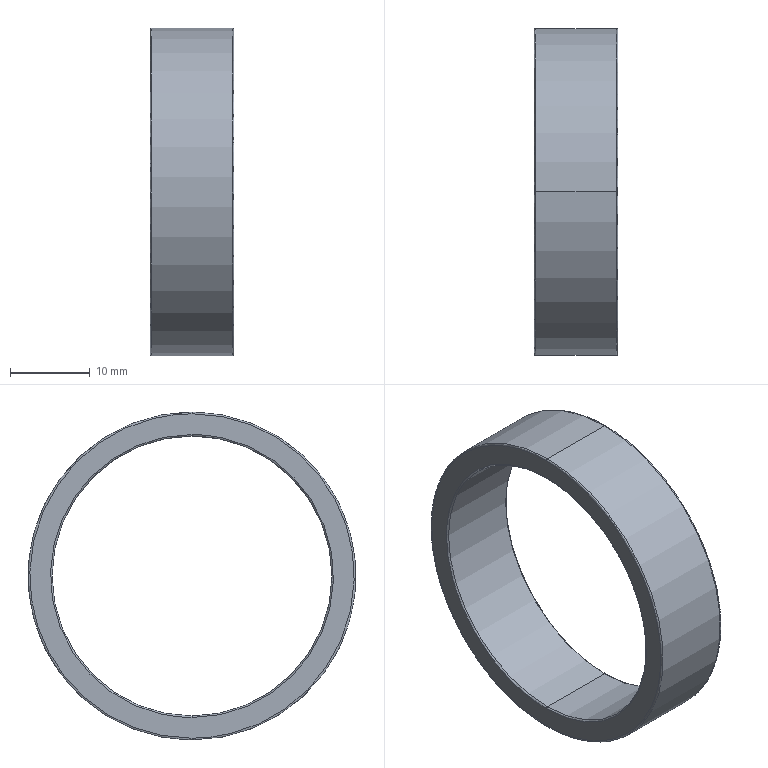Part | SolidWorks | features BaseBody 1 | 1 solid | 14 faces | box 10.5 x 41 x 41 mm | volume 3744 mm3 | spline 8 | cylinder 4 | plane 2 | commonest cylinder face diameters 35.02 x2 41 x2
STEP:
#1=CARTESIAN_POINT('',(10.3,-0.000000002,-20.5));
#2=VERTEX_POINT('',#1);
#3=CARTESIAN_POINT('',(10.3,0.,20.5));
#4=VERTEX_POINT('',#3);
#5=CARTESIAN_POINT('',(10.3,0.,0.));
#6=DIRECTION('',(1.,0.,0.));
#7=DIRECTION('',(0.,1.,0.));
#8=AXIS2_PLACEMENT_3D('',#5,#6,#7);
#9=CIRCLE('',#8,20.5);
#10=EDGE_CURVE('',#2,#4,#9,.T.);
#11=ORIENTED_EDGE('',*,*,#10,.F.);
#12=CARTESIAN_POINT('',(0.2,-0.000000002,-20.5));
#13=VERTEX_POINT('',#12);
#14=CARTESIAN_POINT('',(10.3,0.,-20.5));
#15=DIRECTION('',(-1.,0.,0.));
#16=VECTOR('',#15,1000.);
#17=LINE('',#14,#16);
#18=EDGE_CURVE('',#2,#13,#17,.T.);
#19=ORIENTED_EDGE('',*,*,#18,.T.);
#20=CARTESIAN_POINT('',(0.2,-0.000000001,20.5));
#21=VERTEX_POINT('',#20);
#22=CARTESIAN_POINT('',(0.2,0.,0.));
#23=DIRECTION('',(-1.,0.,0.));
#24=DIRECTION('',(0.,0.,1.));
#25=AXIS2_PLACEMENT_3D('',#22,#23,#24);
#26=CIRCLE('',#25,20.5);
#27=EDGE_CURVE('',#21,#13,#26,.T.);
#28=ORIENTED_EDGE('',*,*,#27,.F.);
#29=CARTESIAN_POINT('',(10.3,0.,20.5));
#30=DIRECTION('',(-1.,0.,0.));
#31=VECTOR('',#30,1000.);
#32=LINE('',#29,#31);
#33=EDGE_CURVE('',#4,#21,#32,.T.);
#34=ORIENTED_EDGE('',*,*,#33,.F.);
#35=EDGE_LOOP('',(#11,#19,#28,#34));
#36=FACE_OUTER_BOUND('',#35,.T.);
#37=CARTESIAN_POINT('',(10.3,0.,0.));
#38=DIRECTION('',(-1.,0.,0.));
#39=DIRECTION('',(0.,0.,1.));
#40=AXIS2_PLACEMENT_3D('',#37,#38,#39);
#41=CYLINDRICAL_SURFACE('',#40,20.5);
#42=ADVANCED_FACE('',(#36),#41,.T.);
#43=CARTESIAN_POINT('',(10.3,-0.000000002,-17.51));
#44=VERTEX_POINT('',#43);
#45=CARTESIAN_POINT('',(10.3,0.,17.51));
#46=VERTEX_POINT('',#45);
#47=CARTESIAN_POINT('',(10.3,0.,0.));
#48=DIRECTION('',(-1.,0.,0.));
#49=DIRECTION('',(0.,-1.,0.));
#50=AXIS2_PLACEMENT_3D('',#47,#48,#49);
#51=CIRCLE('',#50,17.51);
#52=EDGE_CURVE('',#44,#46,#51,.T.);
#53=ORIENTED_EDGE('',*,*,#52,.F.);
#54=CARTESIAN_POINT('',(0.2,-0.000000004,-17.51));
#55=VERTEX_POINT('',#54);
#56=CARTESIAN_POINT('',(10.3,0.,-17.51));
#57=DIRECTION('',(-1.,0.,0.));
#58=VECTOR('',#57,1000.);
#59=LINE('',#56,#58);
#60=EDGE_CURVE('',#44,#55,#59,.T.);
#61=ORIENTED_EDGE('',*,*,#60,.T.);
#62=CARTESIAN_POINT('',(0.2,0.,17.51));
#63=VERTEX_POINT('',#62);
#64=CARTESIAN_POINT('',(0.2,0.,0.));
#65=DIRECTION('',(-1.,0.,0.));
#66=DIRECTION('',(0.,0.,1.));
#67=AXIS2_PLACEMENT_3D('',#64,#65,#66);
#68=CIRCLE('',#67,17.51);
#69=EDGE_CURVE('',#55,#63,#68,.T.);
#70=ORIENTED_EDGE('',*,*,#69,.T.);
#71=CARTESIAN_POINT('',(10.3,0.,17.51));
#72=DIRECTION('',(-1.,0.,0.));
#73=VECTOR('',#72,1000.);
#74=LINE('',#71,#73);
#75=EDGE_CURVE('',#46,#63,#74,.T.);
#76=ORIENTED_EDGE('',*,*,#75,.F.);
#77=EDGE_LOOP('',(#53,#61,#70,#76));
#78=FACE_OUTER_BOUND('',#77,.T.);
#79=CARTESIAN_POINT('',(10.3,0.,0.));
#80=DIRECTION('',(-1.,0.,0.));
#81=DIRECTION('',(0.,0.,1.));
#82=AXIS2_PLACEMENT_3D('',#79,#80,#81);
#83=CYLINDRICAL_SURFACE('',#82,17.51);
#84=ADVANCED_FACE('',(#78),#83,.F.);
#85=CARTESIAN_POINT('',(10.5,0.,20.3));
#86=VERTEX_POINT('',#85);
#87=CARTESIAN_POINT('',(10.5,0.,-20.3));
#88=VERTEX_POINT('',#87);
#89=CARTESIAN_POINT('',(10.5,0.,20.3));
#90=CARTESIAN_POINT('',(10.5,40.6,20.3));
#91=CARTESIAN_POINT('',(10.5,40.6,-20.3));
#92=CARTESIAN_POINT('',(10.5,0.,-20.3));
#93=(BOUNDED_CURVE()B_SPLINE_CURVE(3,(#89,#90,#91,#92),.UNSPECIFIED.,.F.,.F.)B_SPLINE_CURVE_WITH_KNOTS((4,4),(0.,1.),.UNSPECIFIED.)CURVE()GEOMETRIC_REPRESENTATION_ITEM()RATIONAL_B_SPLINE_CURVE((0.9566,0.3189,0.3189,0.9566))REPRESENTATION_ITEM(''));
#94=EDGE_CURVE('',#86,#88,#93,.T.);
#95=ORIENTED_EDGE('',*,*,#94,.T.);
#96=CARTESIAN_POINT('',(10.3,-0.000000002,-20.5));
#97=CARTESIAN_POINT('',(10.417,0.,-20.5));
#98=CARTESIAN_POINT('',(10.5,0.,-20.417));
#99=CARTESIAN_POINT('',(10.5,0.,-20.3));
#100=(BOUNDED_CURVE()B_SPLINE_CURVE(3,(#96,#97,#98,#99),.UNSPECIFIED.,.F.,.F.)B_SPLINE_CURVE_WITH_KNOTS((4,4),(0.06314,0.9369),.UNSPECIFIED.)CURVE()GEOMETRIC_REPRESENTATION_ITEM()RATIONAL_B_SPLINE_CURVE((0.9566,0.7698,0.7698,0.9566))REPRESENTATION_ITEM(''));
#101=EDGE_CURVE('',#2,#88,#100,.T.);
#102=ORIENTED_EDGE('',*,*,#101,.F.);
#103=ORIENTED_EDGE('',*,*,#10,.T.);
#104=CARTESIAN_POINT('',(10.5,0.,20.3));
#105=CARTESIAN_POINT('',(10.5,0.,20.417));
#106=CARTESIAN_POINT('',(10.417,0.,20.5));
#107=CARTESIAN_POINT('',(10.3,0.,20.5));
#108=(BOUNDED_CURVE()B_SPLINE_CURVE(3,(#104,#105,#106,#107),.UNSPECIFIED.,.F.,.F.)B_SPLINE_CURVE_WITH_KNOTS((4,4),(0.06314,0.9369),.UNSPECIFIED.)CURVE()GEOMETRIC_REPRESENTATION_ITEM()RATIONAL_B_SPLINE_CURVE((0.9566,0.7698,0.7698,0.9566))REPRESENTATION_ITEM(''));
#109=EDGE_CURVE('',#86,#4,#108,.T.);
#110=ORIENTED_EDGE('',*,*,#109,.F.);
#111=EDGE_LOOP('',(#95,#102,#103,#110));
#112=FACE_OUTER_BOUND('',#111,.T.);
#113=CARTESIAN_POINT('',(10.499,0.,-20.28));
#114=CARTESIAN_POINT('',(10.499,40.56,-20.28));
#115=CARTESIAN_POINT('',(10.499,40.56,20.28));
#116=CARTESIAN_POINT('',(10.499,0.,20.28));
#117=CARTESIAN_POINT('',(10.513,0.,-20.416));
#118=CARTESIAN_POINT('',(10.513,40.832,-20.416));
#119=CARTESIAN_POINT('',(10.513,40.832,20.416));
#120=CARTESIAN_POINT('',(10.513,0.,20.416));
#121=CARTESIAN_POINT('',(10.416,0.,-20.513));
#122=CARTESIAN_POINT('',(10.416,41.025,-20.513));
#123=CARTESIAN_POINT('',(10.416,41.025,20.513));
#124=CARTESIAN_POINT('',(10.416,0.,20.513));
#125=CARTESIAN_POINT('',(10.28,0.,-20.499));
#126=CARTESIAN_POINT('',(10.28,40.998,-20.499));
#127=CARTESIAN_POINT('',(10.28,40.998,20.499));
#128=CARTESIAN_POINT('',(10.28,0.,20.499));
#129=(BOUNDED_SURFACE()B_SPLINE_SURFACE(3,3,((#113,#114,#115,#116),(#117,#118,#119,#120),(#121,#122,#123,#124),(#125,#126,#127,#128)),.UNSPECIFIED.,.F.,.F.,.T.)B_SPLINE_SURFACE_WITH_KNOTS((4,4),(4,4),(0.,1.),(0.,1.),.UNSPECIFIED.)GEOMETRIC_REPRESENTATION_ITEM()RATIONAL_B_SPLINE_SURFACE(((1.,0.3333,0.3333,1.),(0.7553,0.2518,0.2518,0.7553),(0.7553,0.2518,0.2518,0.7553),(1.,0.3333,0.3333,1.)))REPRESENTATION_ITEM('')SURFACE());
#130=ADVANCED_FACE('',(#112),#129,.T.);
#131=CARTESIAN_POINT('',(10.5,0.,-17.71));
#132=VERTEX_POINT('',#131);
#133=CARTESIAN_POINT('',(10.5,0.,17.71));
#134=VERTEX_POINT('',#133);
#135=CARTESIAN_POINT('',(10.5,0.,-17.71));
#136=CARTESIAN_POINT('',(10.5,-0.3935,-17.71));
#137=CARTESIAN_POINT('',(10.5,-0.9824,-17.69));
#138=CARTESIAN_POINT('',(10.5,-1.667,-17.633));
#139=CARTESIAN_POINT('',(10.5,-2.009,-17.596));
#140=CARTESIAN_POINT('',(10.5,-2.18,-17.575));
#141=CARTESIAN_POINT('',(10.5,-2.266,-17.565));
#142=CARTESIAN_POINT('',(10.5,-2.302,-17.56));
#143=CARTESIAN_POINT('',(10.5,-2.326,-17.557));
#144=CARTESIAN_POINT('',(10.5,-2.337,-17.555));
#145=CARTESIAN_POINT('',(10.5,-2.792,-17.494));
#146=CARTESIAN_POINT('',(10.5,-3.449,-17.381));
#147=CARTESIAN_POINT('',(10.5,-4.207,-17.206));
#148=CARTESIAN_POINT('',(10.5,-4.584,-17.107));
#149=CARTESIAN_POINT('',(10.5,-4.771,-17.055));
#150=CARTESIAN_POINT('',(10.5,-4.865,-17.029));
#151=CARTESIAN_POINT('',(10.5,-4.905,-17.017));
#152=CARTESIAN_POINT('',(10.5,-4.932,-17.009));
#153=CARTESIAN_POINT('',(10.5,-4.944,-17.006));
#154=CARTESIAN_POINT('',(10.5,-5.441,-16.861));
#155=CARTESIAN_POINT('',(10.5,-6.153,-16.62));
#156=CARTESIAN_POINT('',(10.5,-6.963,-16.287));
#157=CARTESIAN_POINT('',(10.5,-7.364,-16.107));
#158=CARTESIAN_POINT('',(10.5,-7.562,-16.014));
#159=CARTESIAN_POINT('',(10.5,-7.662,-15.967));
#160=CARTESIAN_POINT('',(10.5,-7.704,-15.947));
#161=CARTESIAN_POINT('',(10.5,-7.732,-15.933));
#162=CARTESIAN_POINT('',(10.5,-7.745,-15.927));
#163=CARTESIAN_POINT('',(10.5,-8.266,-15.673));
#164=CARTESIAN_POINT('',(10.5,-9.003,-15.269));
#165=CARTESIAN_POINT('',(10.5,-9.827,-14.739));
#166=CARTESIAN_POINT('',(10.5,-10.229,-14.458));
#167=CARTESIAN_POINT('',(10.5,-10.428,-14.314));
#168=CARTESIAN_POINT('',(10.5,-10.527,-14.241));
#169=CARTESIAN_POINT('',(10.5,-10.57,-14.21));
#170=CARTESIAN_POINT('',(10.5,-10.598,-14.189));
#171=CARTESIAN_POINT('',(10.5,-10.611,-14.179));
#172=CARTESIAN_POINT('',(10.5,-10.868,-13.986));
#173=CARTESIAN_POINT('',(10.5,-11.224,-13.705));
#174=CARTESIAN_POINT('',(10.5,-11.626,-13.361));
#175=CARTESIAN_POINT('',(10.5,-11.824,-13.185));
#176=CARTESIAN_POINT('',(10.5,-11.908,-13.109));
#177=CARTESIAN_POINT('',(10.5,-11.964,-13.058));
#178=CARTESIAN_POINT('',(10.5,-11.99,-13.034));
#179=CARTESIAN_POINT('',(10.5,-12.252,-12.792));
#180=CARTESIAN_POINT('',(10.5,-12.592,-12.46));
#181=CARTESIAN_POINT('',(10.5,-12.973,-12.058));
#182=CARTESIAN_POINT('',(10.5,-13.159,-11.853));
#183=CARTESIAN_POINT('',(10.5,-13.238,-11.764));
#184=CARTESIAN_POINT('',(10.5,-13.291,-11.705));
#185=CARTESIAN_POINT('',(10.5,-13.316,-11.676));
#186=CARTESIAN_POINT('',(10.5,-13.56,-11.396));
#187=CARTESIAN_POINT('',(10.5,-13.875,-11.015));
#188=CARTESIAN_POINT('',(10.5,-14.223,-10.554));
#189=CARTESIAN_POINT('',(10.5,-14.393,-10.32));
#190=CARTESIAN_POINT('',(10.5,-14.464,-10.219));
#191=CARTESIAN_POINT('',(10.5,-14.512,-10.152));
#192=CARTESIAN_POINT('',(10.5,-14.534,-10.119));
#193=CARTESIAN_POINT('',(10.5,-14.754,-9.803));
#194=CARTESIAN_POINT('',(10.5,-15.033,-9.373));
#195=CARTESIAN_POINT('',(10.5,-15.337,-8.858));
#196=CARTESIAN_POINT('',(10.5,-15.484,-8.597));
#197=CARTESIAN_POINT('',(10.5,-15.545,-8.485));
#198=CARTESIAN_POINT('',(10.5,-15.586,-8.41));
#199=CARTESIAN_POINT('',(10.5,-15.606,-8.373));
#200=CARTESIAN_POINT('',(10.5,-15.792,-8.023));
#201=CARTESIAN_POINT('',(10.5,-16.027,-7.55));
#202=CARTESIAN_POINT('',(10.5,-16.275,-6.987));
#203=CARTESIAN_POINT('',(10.5,-16.376,-6.743));
#204=CARTESIAN_POINT('',(10.5,-16.443,-6.58));
#205=CARTESIAN_POINT('',(10.5,-16.474,-6.5));
#206=CARTESIAN_POINT('',(10.5,-16.638,-6.08));
#207=CARTESIAN_POINT('',(10.5,-16.818,-5.571));
#208=CARTESIAN_POINT('',(10.5,-17.001,-4.968));
#209=CARTESIAN_POINT('',(10.5,-17.073,-4.708));
#210=CARTESIAN_POINT('',(10.5,-17.12,-4.534));
#211=CARTESIAN_POINT('',(10.5,-17.143,-4.448));
#212=CARTESIAN_POINT('',(10.5,-17.255,-4.005));
#213=CARTESIAN_POINT('',(10.5,-17.374,-3.469));
#214=CARTESIAN_POINT('',(10.5,-17.467,-2.929));
#215=CARTESIAN_POINT('',(10.5,-17.524,-2.568));
#216=CARTESIAN_POINT('',(10.5,-17.549,-2.388));
#217=CARTESIAN_POINT('',(10.5,-17.664,-1.473));
#218=CARTESIAN_POINT('',(10.5,-17.71,-0.7376));
#219=CARTESIAN_POINT('',(10.5,-17.71,0.3688));
#220=CARTESIAN_POINT('',(10.5,-17.693,0.921));
#221=CARTESIAN_POINT('',(10.5,-17.65,1.472));
#222=CARTESIAN_POINT('',(10.5,-17.615,1.839));
#223=CARTESIAN_POINT('',(10.5,-17.595,2.024));
#224=CARTESIAN_POINT('',(10.5,-17.527,2.568));
#225=CARTESIAN_POINT('',(10.5,-17.442,3.11));
#226=CARTESIAN_POINT('',(10.5,-17.313,3.736));
#227=CARTESIAN_POINT('',(10.5,-17.252,4.004));
#228=CARTESIAN_POINT('',(10.5,-17.209,4.182));
#229=CARTESIAN_POINT('',(10.5,-17.187,4.272));
#230=CARTESIAN_POINT('',(10.5,-17.076,4.709));
#231=CARTESIAN_POINT('',(10.5,-16.928,5.228));
#232=CARTESIAN_POINT('',(10.5,-16.727,5.825));
#233=CARTESIAN_POINT('',(10.5,-16.634,6.078));
#234=CARTESIAN_POINT('',(10.5,-16.572,6.247));
#235=CARTESIAN_POINT('',(10.5,-16.539,6.334));
#236=CARTESIAN_POINT('',(10.5,-16.379,6.744));
#237=CARTESIAN_POINT('',(10.5,-16.174,7.23));
#238=CARTESIAN_POINT('',(10.5,-15.908,7.786));
#239=CARTESIAN_POINT('',(10.5,-15.77,8.061));
#240=CARTESIAN_POINT('',(10.5,-15.709,8.178));
#241=CARTESIAN_POINT('',(10.5,-15.668,8.256));
#242=CARTESIAN_POINT('',(10.5,-15.647,8.296));
#243=CARTESIAN_POINT('',(10.5,-15.466,8.636));
#244=CARTESIAN_POINT('',(10.5,-15.211,9.081));
#245=CARTESIAN_POINT('',(10.5,-14.892,9.587));
#246=CARTESIAN_POINT('',(10.5,-14.727,9.837));
#247=CARTESIAN_POINT('',(10.5,-14.656,9.943));
#248=CARTESIAN_POINT('',(10.5,-14.607,10.014));
#249=CARTESIAN_POINT('',(10.5,-14.582,10.05));
#250=CARTESIAN_POINT('',(10.5,-14.371,10.355));
#251=CARTESIAN_POINT('',(10.5,-14.078,10.754));
#252=CARTESIAN_POINT('',(10.5,-13.717,11.204));
#253=CARTESIAN_POINT('',(10.5,-13.532,11.426));
#254=CARTESIAN_POINT('',(10.5,-13.451,11.52));
#255=CARTESIAN_POINT('',(10.5,-13.397,11.583));
#256=CARTESIAN_POINT('',(10.5,-13.369,11.615));
#257=CARTESIAN_POINT('',(10.5,-13.135,11.884));
#258=CARTESIAN_POINT('',(10.5,-12.813,12.233));
#259=CARTESIAN_POINT('',(10.5,-12.422,12.625));
#260=CARTESIAN_POINT('',(10.5,-12.222,12.817));
#261=CARTESIAN_POINT('',(10.5,-12.136,12.899));
#262=CARTESIAN_POINT('',(10.5,-12.078,12.953));
#263=CARTESIAN_POINT('',(10.5,-12.047,12.981));
#264=CARTESIAN_POINT('',(10.5,-11.797,13.212));
#265=CARTESIAN_POINT('',(10.5,-11.457,13.511));
#266=CARTESIAN_POINT('',(10.5,-11.046,13.845));
#267=CARTESIAN_POINT('',(10.5,-10.837,14.008));
#268=CARTESIAN_POINT('',(10.5,-10.732,14.088));
#269=CARTESIAN_POINT('',(10.5,-10.686,14.122));
#270=CARTESIAN_POINT('',(10.5,-10.656,14.145));
#271=CARTESIAN_POINT('',(10.5,-10.64,14.157));
#272=CARTESIAN_POINT('',(10.5,-10.176,14.505));
#273=CARTESIAN_POINT('',(10.5,-9.481,14.977));
#274=CARTESIAN_POINT('',(10.5,-8.633,15.468));
#275=CARTESIAN_POINT('',(10.5,-8.2,15.698));
#276=CARTESIAN_POINT('',(10.5,-7.981,15.81));
#277=CARTESIAN_POINT('',(10.5,-7.871,15.865));
#278=CARTESIAN_POINT('',(10.5,-7.824,15.888));
#279=CARTESIAN_POINT('',(10.5,-7.792,15.904));
#280=CARTESIAN_POINT('',(10.5,-7.775,15.912));
#281=CARTESIAN_POINT('',(10.5,-7.309,16.139));
#282=CARTESIAN_POINT('',(10.5,-6.62,16.44));
#283=CARTESIAN_POINT('',(10.5,-5.796,16.738));
#284=CARTESIAN_POINT('',(10.5,-5.379,16.874));
#285=CARTESIAN_POINT('',(10.5,-5.169,16.939));
#286=CARTESIAN_POINT('',(10.5,-5.064,16.971));
#287=CARTESIAN_POINT('',(10.5,-5.019,16.984));
#288=CARTESIAN_POINT('',(10.5,-4.989,16.993));
#289=CARTESIAN_POINT('',(10.5,-4.972,16.998));
#290=CARTESIAN_POINT('',(10.5,-4.531,17.126));
#291=CARTESIAN_POINT('',(10.5,-3.885,17.289));
#292=CARTESIAN_POINT('',(10.5,-3.121,17.435));
#293=CARTESIAN_POINT('',(10.5,-2.737,17.498));
#294=CARTESIAN_POINT('',(10.5,-2.544,17.526));
#295=CARTESIAN_POINT('',(10.5,-2.447,17.54));
#296=CARTESIAN_POINT('',(10.5,-2.406,17.546));
#297=CARTESIAN_POINT('',(10.5,-2.378,17.55));
#298=CARTESIAN_POINT('',(10.5,-2.363,17.552));
#299=CARTESIAN_POINT('',(10.5,-1.571,17.658));
#300=CARTESIAN_POINT('',(10.5,-0.7873,17.71));
#301=CARTESIAN_POINT('',(10.5,0.,17.71));
#302=B_SPLINE_CURVE_WITH_KNOTS('',3,(#135,#136,#137,#138,#139,#140,#141,#142,#143,#144,#145,#146,#147,#148,#149,#150,#151,#152,#153,#154,#155,#156,#157,#158,#159,#160,#161,#162,#163,#164,#165,#166,#167,#168,#169,#170,#171,#172,#173,#174,#175,#176,#177,#178,#179,#180,#181,#182,#183,#184,#185,#186,#187,#188,#189,#190,#191,#192,#193,#194,#195,#196,#197,#198,#199,#200,#201,#202,#203,#204,#205,#206,#207,#208,#209,#210,#211,#212,#213,#214,#215,#216,#217,#218,#219,#220,#221,#222,#223,#224,#225,#226,#227,#228,#229,#230,#231,#232,#233,#234,#235,#236,#237,#238,#239,#240,#241,#242,#243,#244,#245,#246,#247,#248,#249,#250,#251,#252,#253,#254,#255,#256,#257,#258,#259,#260,#261,#262,#263,#264,#265,#266,#267,#268,#269,#270,#271,#272,#273,#274,#275,#276,#277,#278,#279,#280,#281,#282,#283,#284,#285,#286,#287,#288,#289,#290,#291,#292,#293,#294,#295,#296,#297,#298,#299,#300,#301),.UNSPECIFIED.,.F.,.F.,(4,1,1,1,1,1,2,2,1,1,1,1,1,2,2,1,1,1,1,1,2,2,1,1,1,1,1,2,2,1,1,1,2,2,1,1,1,2,2,1,1,1,2,2,1,1,1,2,2,1,1,2,2,1,1,2,2,1,2,2,2,1,2,2,1,1,2,2,1,1,2,2,1,1,1,2,2,1,1,1,2,2,1,1,1,2,2,1,1,1,2,2,1,1,1,1,2,2,1,1,1,1,1,2,2,1,1,1,1,1,2,2,1,1,1,1,1,2,2,4),(0.,0.03125,0.04688,0.05469,0.05859,0.06055,0.06152,0.0625,0.09375,0.1094,0.1172,0.1211,0.123,0.124,0.125,0.1563,0.1719,0.1797,0.1836,0.1855,0.1865,0.1875,0.2188,0.2344,0.2422,0.2461,0.248,0.249,0.25,0.2656,0.2734,0.2773,0.2793,0.2813,0.2969,0.3047,0.3086,0.3105,0.3125,0.3281,0.3359,0.3398,0.3418,0.3438,0.3594,0.3672,0.3711,0.373,0.375,0.3906,0.3984,0.4023,0.4063,0.4219,0.4297,0.4336,0.4375,0.4531,0.4609,0.4688,0.5,0.5156,0.5234,0.5313,0.5469,0.5547,0.5586,0.5625,0.5781,0.5859,0.5898,0.5938,0.6094,0.6172,0.6211,0.623,0.625,0.6406,0.6484,0.6523,0.6543,0.6563,0.6719,0.6797,0.6836,0.6855,0.6875,0.7031,0.7109,0.7148,0.7168,0.7188,0.7344,0.7422,0.7461,0.748,0.749,0.75,0.7813,0.7969,0.8047,0.8086,0.8105,0.8115,0.8125,0.8438,0.8594,0.8672,0.8711,0.873,0.874,0.875,0.9063,0.9219,0.9297,0.9336,0.9355,0.9365,0.9375,1.),.UNSPECIFIED.);
#303=EDGE_CURVE('',#132,#134,#302,.T.);
#304=ORIENTED_EDGE('',*,*,#303,.T.);
#305=CARTESIAN_POINT('',(10.5,0.,17.71));
#306=CARTESIAN_POINT('',(10.5,0.3935,17.71));
#307=CARTESIAN_POINT('',(10.5,0.9824,17.69));
#308=CARTESIAN_POINT('',(10.5,1.667,17.633));
#309=CARTESIAN_POINT('',(10.5,2.009,17.596));
#310=CARTESIAN_POINT('',(10.5,2.18,17.575));
#311=CARTESIAN_POINT('',(10.5,2.266,17.565));
#312=CARTESIAN_POINT('',(10.5,2.302,17.56));
#313=CARTESIAN_POINT('',(10.5,2.326,17.557));
#314=CARTESIAN_POINT('',(10.5,2.337,17.555));
#315=CARTESIAN_POINT('',(10.5,2.792,17.494));
#316=CARTESIAN_POINT('',(10.5,3.449,17.381));
#317=CARTESIAN_POINT('',(10.5,4.207,17.206));
#318=CARTESIAN_POINT('',(10.5,4.584,17.107));
#319=CARTESIAN_POINT('',(10.5,4.771,17.055));
#320=CARTESIAN_POINT('',(10.5,4.865,17.029));
#321=CARTESIAN_POINT('',(10.5,4.905,17.017));
#322=CARTESIAN_POINT('',(10.5,4.932,17.009));
#323=CARTESIAN_POINT('',(10.5,4.944,17.006));
#324=CARTESIAN_POINT('',(10.5,5.441,16.861));
#325=CARTESIAN_POINT('',(10.5,6.153,16.62));
#326=CARTESIAN_POINT('',(10.5,6.963,16.287));
#327=CARTESIAN_POINT('',(10.5,7.364,16.107));
#328=CARTESIAN_POINT('',(10.5,7.562,16.014));
#329=CARTESIAN_POINT('',(10.5,7.662,15.967));
#330=CARTESIAN_POINT('',(10.5,7.704,15.947));
#331=CARTESIAN_POINT('',(10.5,7.732,15.933));
#332=CARTESIAN_POINT('',(10.5,7.745,15.927));
#333=CARTESIAN_POINT('',(10.5,8.266,15.673));
#334=CARTESIAN_POINT('',(10.5,9.003,15.269));
#335=CARTESIAN_POINT('',(10.5,9.827,14.739));
#336=CARTESIAN_POINT('',(10.5,10.229,14.458));
#337=CARTESIAN_POINT('',(10.5,10.428,14.314));
#338=CARTESIAN_POINT('',(10.5,10.527,14.241));
#339=CARTESIAN_POINT('',(10.5,10.57,14.21));
#340=CARTESIAN_POINT('',(10.5,10.598,14.189));
#341=CARTESIAN_POINT('',(10.5,10.611,14.179));
#342=CARTESIAN_POINT('',(10.5,10.868,13.986));
#343=CARTESIAN_POINT('',(10.5,11.224,13.705));
#344=CARTESIAN_POINT('',(10.5,11.626,13.361));
#345=CARTESIAN_POINT('',(10.5,11.824,13.185));
#346=CARTESIAN_POINT('',(10.5,11.908,13.109));
#347=CARTESIAN_POINT('',(10.5,11.964,13.058));
#348=CARTESIAN_POINT('',(10.5,11.99,13.034));
#349=CARTESIAN_POINT('',(10.5,12.252,12.792));
#350=CARTESIAN_POINT('',(10.5,12.592,12.46));
#351=CARTESIAN_POINT('',(10.5,12.973,12.058));
#352=CARTESIAN_POINT('',(10.5,13.159,11.853));
#353=CARTESIAN_POINT('',(10.5,13.238,11.764));
#354=CARTESIAN_POINT('',(10.5,13.291,11.705));
#355=CARTESIAN_POINT('',(10.5,13.316,11.676));
#356=CARTESIAN_POINT('',(10.5,13.56,11.396));
#357=CARTESIAN_POINT('',(10.5,13.875,11.015));
#358=CARTESIAN_POINT('',(10.5,14.223,10.554));
#359=CARTESIAN_POINT('',(10.5,14.393,10.32));
#360=CARTESIAN_POINT('',(10.5,14.464,10.219));
#361=CARTESIAN_POINT('',(10.5,14.512,10.152));
#362=CARTESIAN_POINT('',(10.5,14.534,10.119));
#363=CARTESIAN_POINT('',(10.5,14.754,9.803));
#364=CARTESIAN_POINT('',(10.5,15.033,9.373));
#365=CARTESIAN_POINT('',(10.5,15.337,8.858));
#366=CARTESIAN_POINT('',(10.5,15.484,8.597));
#367=CARTESIAN_POINT('',(10.5,15.545,8.485));
#368=CARTESIAN_POINT('',(10.5,15.586,8.41));
#369=CARTESIAN_POINT('',(10.5,15.606,8.373));
#370=CARTESIAN_POINT('',(10.5,15.792,8.023));
#371=CARTESIAN_POINT('',(10.5,16.027,7.55));
#372=CARTESIAN_POINT('',(10.5,16.275,6.987));
#373=CARTESIAN_POINT('',(10.5,16.376,6.743));
#374=CARTESIAN_POINT('',(10.5,16.443,6.58));
#375=CARTESIAN_POINT('',(10.5,16.474,6.5));
#376=CARTESIAN_POINT('',(10.5,16.638,6.08));
#377=CARTESIAN_POINT('',(10.5,16.818,5.571));
#378=CARTESIAN_POINT('',(10.5,17.001,4.968));
#379=CARTESIAN_POINT('',(10.5,17.073,4.708));
#380=CARTESIAN_POINT('',(10.5,17.12,4.534));
#381=CARTESIAN_POINT('',(10.5,17.143,4.448));
#382=CARTESIAN_POINT('',(10.5,17.255,4.005));
#383=CARTESIAN_POINT('',(10.5,17.374,3.469));
#384=CARTESIAN_POINT('',(10.5,17.467,2.929));
#385=CARTESIAN_POINT('',(10.5,17.524,2.568));
#386=CARTESIAN_POINT('',(10.5,17.549,2.388));
#387=CARTESIAN_POINT('',(10.5,17.664,1.473));
#388=CARTESIAN_POINT('',(10.5,17.71,0.7376));
#389=CARTESIAN_POINT('',(10.5,17.71,-0.3688));
#390=CARTESIAN_POINT('',(10.5,17.693,-0.921));
#391=CARTESIAN_POINT('',(10.5,17.65,-1.472));
#392=CARTESIAN_POINT('',(10.5,17.615,-1.839));
#393=CARTESIAN_POINT('',(10.5,17.595,-2.024));
#394=CARTESIAN_POINT('',(10.5,17.527,-2.568));
#395=CARTESIAN_POINT('',(10.5,17.442,-3.11));
#396=CARTESIAN_POINT('',(10.5,17.313,-3.736));
#397=CARTESIAN_POINT('',(10.5,17.252,-4.004));
#398=CARTESIAN_POINT('',(10.5,17.209,-4.182));
#399=CARTESIAN_POINT('',(10.5,17.187,-4.272));
#400=CARTESIAN_POINT('',(10.5,17.076,-4.709));
#401=CARTESIAN_POINT('',(10.5,16.928,-5.228));
#402=CARTESIAN_POINT('',(10.5,16.727,-5.825));
#403=CARTESIAN_POINT('',(10.5,16.634,-6.078));
#404=CARTESIAN_POINT('',(10.5,16.572,-6.247));
#405=CARTESIAN_POINT('',(10.5,16.539,-6.334));
#406=CARTESIAN_POINT('',(10.5,16.379,-6.744));
#407=CARTESIAN_POINT('',(10.5,16.174,-7.23));
#408=CARTESIAN_POINT('',(10.5,15.908,-7.786));
#409=CARTESIAN_POINT('',(10.5,15.77,-8.061));
#410=CARTESIAN_POINT('',(10.5,15.709,-8.178));
#411=CARTESIAN_POINT('',(10.5,15.668,-8.256));
#412=CARTESIAN_POINT('',(10.5,15.647,-8.296));
#413=CARTESIAN_POINT('',(10.5,15.466,-8.636));
#414=CARTESIAN_POINT('',(10.5,15.211,-9.081));
#415=CARTESIAN_POINT('',(10.5,14.892,-9.587));
#416=CARTESIAN_POINT('',(10.5,14.727,-9.837));
#417=CARTESIAN_POINT('',(10.5,14.656,-9.943));
#418=CARTESIAN_POINT('',(10.5,14.607,-10.014));
#419=CARTESIAN_POINT('',(10.5,14.582,-10.05));
#420=CARTESIAN_POINT('',(10.5,14.371,-10.355));
#421=CARTESIAN_POINT('',(10.5,14.078,-10.754));
#422=CARTESIAN_POINT('',(10.5,13.717,-11.204));
#423=CARTESIAN_POINT('',(10.5,13.532,-11.426));
#424=CARTESIAN_POINT('',(10.5,13.451,-11.52));
#425=CARTESIAN_POINT('',(10.5,13.397,-11.583));
#426=CARTESIAN_POINT('',(10.5,13.369,-11.615));
#427=CARTESIAN_POINT('',(10.5,13.135,-11.884));
#428=CARTESIAN_POINT('',(10.5,12.813,-12.233));
#429=CARTESIAN_POINT('',(10.5,12.422,-12.625));
#430=CARTESIAN_POINT('',(10.5,12.222,-12.817));
#431=CARTESIAN_POINT('',(10.5,12.136,-12.899));
#432=CARTESIAN_POINT('',(10.5,12.078,-12.953));
#433=CARTESIAN_POINT('',(10.5,12.047,-12.981));
#434=CARTESIAN_POINT('',(10.5,11.797,-13.212));
#435=CARTESIAN_POINT('',(10.5,11.457,-13.511));
#436=CARTESIAN_POINT('',(10.5,11.046,-13.845));
#437=CARTESIAN_POINT('',(10.5,10.837,-14.008));
#438=CARTESIAN_POINT('',(10.5,10.732,-14.088));
#439=CARTESIAN_POINT('',(10.5,10.686,-14.122));
#440=CARTESIAN_POINT('',(10.5,10.656,-14.145));
#441=CARTESIAN_POINT('',(10.5,10.64,-14.157));
#442=CARTESIAN_POINT('',(10.5,10.176,-14.505));
#443=CARTESIAN_POINT('',(10.5,9.481,-14.977));
#444=CARTESIAN_POINT('',(10.5,8.633,-15.468));
#445=CARTESIAN_POINT('',(10.5,8.2,-15.698));
#446=CARTESIAN_POINT('',(10.5,7.981,-15.81));
#447=CARTESIAN_POINT('',(10.5,7.871,-15.865));
#448=CARTESIAN_POINT('',(10.5,7.824,-15.888));
#449=CARTESIAN_POINT('',(10.5,7.792,-15.904));
#450=CARTESIAN_POINT('',(10.5,7.775,-15.912));
#451=CARTESIAN_POINT('',(10.5,7.309,-16.139));
#452=CARTESIAN_POINT('',(10.5,6.62,-16.44));
#453=CARTESIAN_POINT('',(10.5,5.796,-16.738));
#454=CARTESIAN_POINT('',(10.5,5.379,-16.874));
#455=CARTESIAN_POINT('',(10.5,5.169,-16.939));
#456=CARTESIAN_POINT('',(10.5,5.064,-16.971));
#457=CARTESIAN_POINT('',(10.5,5.019,-16.984));
#458=CARTESIAN_POINT('',(10.5,4.989,-16.993));
#459=CARTESIAN_POINT('',(10.5,4.972,-16.998));
#460=CARTESIAN_POINT('',(10.5,4.531,-17.126));
#461=CARTESIAN_POINT('',(10.5,3.885,-17.289));
#462=CARTESIAN_POINT('',(10.5,3.121,-17.435));
#463=CARTESIAN_POINT('',(10.5,2.737,-17.498));
#464=CARTESIAN_POINT('',(10.5,2.544,-17.526));
#465=CARTESIAN_POINT('',(10.5,2.447,-17.54));
#466=CARTESIAN_POINT('',(10.5,2.406,-17.546));
#467=CARTESIAN_POINT('',(10.5,2.378,-17.55));
#468=CARTESIAN_POINT('',(10.5,2.363,-17.552));
#469=CARTESIAN_POINT('',(10.5,1.571,-17.658));
#470=CARTESIAN_POINT('',(10.5,0.7873,-17.71));
#471=CARTESIAN_POINT('',(10.5,0.,-17.71));
#472=B_SPLINE_CURVE_WITH_KNOTS('',3,(#305,#306,#307,#308,#309,#310,#311,#312,#313,#314,#315,#316,#317,#318,#319,#320,#321,#322,#323,#324,#325,#326,#327,#328,#329,#330,#331,#332,#333,#334,#335,#336,#337,#338,#339,#340,#341,#342,#343,#344,#345,#346,#347,#348,#349,#350,#351,#352,#353,#354,#355,#356,#357,#358,#359,#360,#361,#362,#363,#364,#365,#366,#367,#368,#369,#370,#371,#372,#373,#374,#375,#376,#377,#378,#379,#380,#381,#382,#383,#384,#385,#386,#387,#388,#389,#390,#391,#392,#393,#394,#395,#396,#397,#398,#399,#400,#401,#402,#403,#404,#405,#406,#407,#408,#409,#410,#411,#412,#413,#414,#415,#416,#417,#418,#419,#420,#421,#422,#423,#424,#425,#426,#427,#428,#429,#430,#431,#432,#433,#434,#435,#436,#437,#438,#439,#440,#441,#442,#443,#444,#445,#446,#447,#448,#449,#450,#451,#452,#453,#454,#455,#456,#457,#458,#459,#460,#461,#462,#463,#464,#465,#466,#467,#468,#469,#470,#471),.UNSPECIFIED.,.F.,.F.,(4,1,1,1,1,1,2,2,1,1,1,1,1,2,2,1,1,1,1,1,2,2,1,1,1,1,1,2,2,1,1,1,2,2,1,1,1,2,2,1,1,1,2,2,1,1,1,2,2,1,1,2,2,1,1,2,2,1,2,2,2,1,2,2,1,1,2,2,1,1,2,2,1,1,1,2,2,1,1,1,2,2,1,1,1,2,2,1,1,1,2,2,1,1,1,1,2,2,1,1,1,1,1,2,2,1,1,1,1,1,2,2,1,1,1,1,1,2,2,4),(0.,0.03125,0.04687,0.05469,0.05859,0.06055,0.06152,0.0625,0.09375,0.1094,0.1172,0.1211,0.123,0.124,0.125,0.1562,0.1719,0.1797,0.1836,0.1855,0.1865,0.1875,0.2187,0.2344,0.2422,0.2461,0.248,0.249,0.25,0.2656,0.2734,0.2773,0.2793,0.2812,0.2969,0.3047,0.3086,0.3105,0.3125,0.3281,0.3359,0.3398,0.3418,0.3437,0.3594,0.3672,0.3711,0.373,0.375,0.3906,0.3984,0.4023,0.4062,0.4219,0.4297,0.4336,0.4375,0.4531,0.4609,0.4687,0.5,0.5156,0.5234,0.5312,0.5469,0.5547,0.5586,0.5625,0.5781,0.5859,0.5898,0.5937,0.6094,0.6172,0.6211,0.623,0.625,0.6406,0.6484,0.6523,0.6543,0.6562,0.6719,0.6797,0.6836,0.6855,0.6875,0.7031,0.7109,0.7148,0.7168,0.7187,0.7344,0.7422,0.7461,0.748,0.749,0.75,0.7812,0.7969,0.8047,0.8086,0.8105,0.8115,0.8125,0.8437,0.8594,0.8672,0.8711,0.873,0.874,0.875,0.9062,0.9219,0.9297,0.9336,0.9355,0.9365,0.9375,1.),.UNSPECIFIED.);
#473=EDGE_CURVE('',#134,#132,#472,.T.);
#474=ORIENTED_EDGE('',*,*,#473,.T.);
#475=EDGE_LOOP('',(#304,#474));
#476=FACE_BOUND('',#475,.T.);
#477=ORIENTED_EDGE('',*,*,#94,.F.);
#478=CARTESIAN_POINT('',(10.5,0.,20.3));
#479=CARTESIAN_POINT('',(10.5,-0.451,20.3));
#480=CARTESIAN_POINT('',(10.5,-1.126,20.278));
#481=CARTESIAN_POINT('',(10.5,-1.911,20.212));
#482=CARTESIAN_POINT('',(10.5,-2.303,20.169));
#483=CARTESIAN_POINT('',(10.5,-2.499,20.146));
#484=CARTESIAN_POINT('',(10.5,-2.597,20.133));
#485=CARTESIAN_POINT('',(10.5,-2.639,20.128));
#486=CARTESIAN_POINT('',(10.5,-2.667,20.124));
#487=CARTESIAN_POINT('',(10.5,-2.679,20.122));
#488=CARTESIAN_POINT('',(10.5,-3.201,20.053));
#489=CARTESIAN_POINT('',(10.5,-3.954,19.923));
#490=CARTESIAN_POINT('',(10.5,-4.822,19.722));
#491=CARTESIAN_POINT('',(10.5,-5.254,19.609));
#492=CARTESIAN_POINT('',(10.5,-5.469,19.55));
#493=CARTESIAN_POINT('',(10.5,-5.577,19.519));
#494=CARTESIAN_POINT('',(10.5,-5.623,19.506));
#495=CARTESIAN_POINT('',(10.5,-5.653,19.497));
#496=CARTESIAN_POINT('',(10.5,-5.667,19.493));
#497=CARTESIAN_POINT('',(10.5,-6.237,19.327));
#498=CARTESIAN_POINT('',(10.5,-7.053,19.051));
#499=CARTESIAN_POINT('',(10.5,-7.982,18.669));
#500=CARTESIAN_POINT('',(10.5,-8.441,18.463));
#501=CARTESIAN_POINT('',(10.5,-8.668,18.356));
#502=CARTESIAN_POINT('',(10.5,-8.782,18.302));
#503=CARTESIAN_POINT('',(10.5,-8.831,18.279));
#504=CARTESIAN_POINT('',(10.5,-8.863,18.263));
#505=CARTESIAN_POINT('',(10.5,-8.878,18.256));
#506=CARTESIAN_POINT('',(10.5,-9.177,18.11));
#507=CARTESIAN_POINT('',(10.5,-9.593,17.895));
#508=CARTESIAN_POINT('',(10.5,-10.07,17.627));
#509=CARTESIAN_POINT('',(10.5,-10.307,17.489));
#510=CARTESIAN_POINT('',(10.5,-10.407,17.429));
#511=CARTESIAN_POINT('',(10.5,-10.475,17.389));
#512=CARTESIAN_POINT('',(10.5,-10.506,17.37));
#513=CARTESIAN_POINT('',(10.5,-10.823,17.177));
#514=CARTESIAN_POINT('',(10.5,-11.24,16.91));
#515=CARTESIAN_POINT('',(10.5,-11.714,16.581));
#516=CARTESIAN_POINT('',(10.5,-11.948,16.412));
#517=CARTESIAN_POINT('',(10.5,-12.048,16.339));
#518=CARTESIAN_POINT('',(10.5,-12.114,16.289));
#519=CARTESIAN_POINT('',(10.5,-12.145,16.266));
#520=CARTESIAN_POINT('',(10.5,-12.457,16.032));
#521=CARTESIAN_POINT('',(10.5,-12.865,15.709));
#522=CARTESIAN_POINT('',(10.5,-13.326,15.315));
#523=CARTESIAN_POINT('',(10.5,-13.553,15.114));
#524=CARTESIAN_POINT('',(10.5,-13.649,15.026));
#525=CARTESIAN_POINT('',(10.5,-13.714,14.968));
#526=CARTESIAN_POINT('',(10.5,-13.744,14.94));
#527=CARTESIAN_POINT('',(10.5,-14.044,14.662));
#528=CARTESIAN_POINT('',(10.5,-14.434,14.282));
#529=CARTESIAN_POINT('',(10.5,-14.87,13.821));
#530=CARTESIAN_POINT('',(10.5,-15.084,13.586));
#531=CARTESIAN_POINT('',(10.5,-15.174,13.484));
#532=CARTESIAN_POINT('',(10.5,-15.235,13.416));
#533=CARTESIAN_POINT('',(10.5,-15.263,13.384));
#534=CARTESIAN_POINT('',(10.5,-15.543,13.063));
#535=CARTESIAN_POINT('',(10.5,-15.904,12.625));
#536=CARTESIAN_POINT('',(10.5,-16.303,12.098));
#537=CARTESIAN_POINT('',(10.5,-16.497,11.83));
#538=CARTESIAN_POINT('',(10.5,-16.579,11.714));
#539=CARTESIAN_POINT('',(10.5,-16.634,11.636));
#540=CARTESIAN_POINT('',(10.5,-16.66,11.599));
#541=CARTESIAN_POINT('',(10.5,-16.911,11.236));
#542=CARTESIAN_POINT('',(10.5,-17.232,10.744));
#543=CARTESIAN_POINT('',(10.5,-17.58,10.154));
#544=CARTESIAN_POINT('',(10.5,-17.748,9.855));
#545=CARTESIAN_POINT('',(10.5,-17.819,9.726));
#546=CARTESIAN_POINT('',(10.5,-17.865,9.639));
#547=CARTESIAN_POINT('',(10.5,-17.888,9.597));
#548=CARTESIAN_POINT('',(10.5,-18.102,9.197));
#549=CARTESIAN_POINT('',(10.5,-18.37,8.655));
#550=CARTESIAN_POINT('',(10.5,-18.655,8.009));
#551=CARTESIAN_POINT('',(10.5,-18.771,7.729));
#552=CARTESIAN_POINT('',(10.5,-18.847,7.542));
#553=CARTESIAN_POINT('',(10.5,-18.884,7.45));
#554=CARTESIAN_POINT('',(10.5,-19.071,6.969));
#555=CARTESIAN_POINT('',(10.5,-19.277,6.386));
#556=CARTESIAN_POINT('',(10.5,-19.487,5.695));
#557=CARTESIAN_POINT('',(10.5,-19.57,5.396));
#558=CARTESIAN_POINT('',(10.5,-19.624,5.197));
#559=CARTESIAN_POINT('',(10.5,-19.65,5.099));
#560=CARTESIAN_POINT('',(10.5,-19.779,4.59));
#561=CARTESIAN_POINT('',(10.5,-19.914,3.977));
#562=CARTESIAN_POINT('',(10.5,-20.022,3.358));
#563=CARTESIAN_POINT('',(10.5,-20.087,2.944));
#564=CARTESIAN_POINT('',(10.5,-20.116,2.737));
#565=CARTESIAN_POINT('',(10.5,-20.247,1.689));
#566=CARTESIAN_POINT('',(10.5,-20.3,0.8455));
#567=CARTESIAN_POINT('',(10.5,-20.3,-0.4227));
#568=CARTESIAN_POINT('',(10.5,-20.28,-1.056));
#569=CARTESIAN_POINT('',(10.5,-20.231,-1.687));
#570=CARTESIAN_POINT('',(10.5,-20.191,-2.108));
#571=CARTESIAN_POINT('',(10.5,-20.168,-2.32));
#572=CARTESIAN_POINT('',(10.5,-20.09,-2.944));
#573=CARTESIAN_POINT('',(10.5,-19.992,-3.565));
#574=CARTESIAN_POINT('',(10.5,-19.845,-4.283));
#575=CARTESIAN_POINT('',(10.5,-19.775,-4.589));
#576=CARTESIAN_POINT('',(10.5,-19.726,-4.793));
#577=CARTESIAN_POINT('',(10.5,-19.701,-4.897));
#578=CARTESIAN_POINT('',(10.5,-19.574,-5.397));
#579=CARTESIAN_POINT('',(10.5,-19.403,-5.992));
#580=CARTESIAN_POINT('',(10.5,-19.173,-6.676));
#581=CARTESIAN_POINT('',(10.5,-19.05,-7.016));
#582=CARTESIAN_POINT('',(10.5,-18.995,-7.161));
#583=CARTESIAN_POINT('',(10.5,-18.958,-7.258));
#584=CARTESIAN_POINT('',(10.5,-18.939,-7.307));
#585=CARTESIAN_POINT('',(10.5,-18.775,-7.73));
#586=CARTESIAN_POINT('',(10.5,-18.539,-8.288));
#587=CARTESIAN_POINT('',(10.5,-18.235,-8.925));
#588=CARTESIAN_POINT('',(10.5,-18.076,-9.24));
#589=CARTESIAN_POINT('',(10.5,-18.006,-9.374));
#590=CARTESIAN_POINT('',(10.5,-17.959,-9.464));
#591=CARTESIAN_POINT('',(10.5,-17.935,-9.51));
#592=CARTESIAN_POINT('',(10.5,-17.727,-9.899));
#593=CARTESIAN_POINT('',(10.5,-17.436,-10.409));
#594=CARTESIAN_POINT('',(10.5,-17.07,-10.989));
#595=CARTESIAN_POINT('',(10.5,-16.881,-11.275));
#596=CARTESIAN_POINT('',(10.5,-16.799,-11.397));
#597=CARTESIAN_POINT('',(10.5,-16.744,-11.478));
#598=CARTESIAN_POINT('',(10.5,-16.715,-11.52));
#599=CARTESIAN_POINT('',(10.5,-16.472,-11.87));
#600=CARTESIAN_POINT('',(10.5,-16.137,-12.327));
#601=CARTESIAN_POINT('',(10.5,-15.723,-12.843));
#602=CARTESIAN_POINT('',(10.5,-15.511,-13.097));
#603=CARTESIAN_POINT('',(10.5,-15.418,-13.205));
#604=CARTESIAN_POINT('',(10.5,-15.357,-13.277));
#605=CARTESIAN_POINT('',(10.5,-15.324,-13.314));
#606=CARTESIAN_POINT('',(10.5,-15.056,-13.622));
#607=CARTESIAN_POINT('',(10.5,-14.687,-14.022));
#608=CARTESIAN_POINT('',(10.5,-14.238,-14.471));
#609=CARTESIAN_POINT('',(10.5,-14.009,-14.692));
#610=CARTESIAN_POINT('',(10.5,-13.91,-14.785));
#611=CARTESIAN_POINT('',(10.5,-13.844,-14.847));
#612=CARTESIAN_POINT('',(10.5,-13.809,-14.879));
#613=CARTESIAN_POINT('',(10.5,-13.523,-15.144));
#614=CARTESIAN_POINT('',(10.5,-13.132,-15.487));
#615=CARTESIAN_POINT('',(10.5,-12.661,-15.87));
#616=CARTESIAN_POINT('',(10.5,-12.422,-16.056));
#617=CARTESIAN_POINT('',(10.5,-12.318,-16.135));
#618=CARTESIAN_POINT('',(10.5,-12.249,-16.188));
#619=CARTESIAN_POINT('',(10.5,-12.213,-16.215));
#620=CARTESIAN_POINT('',(10.5,-11.916,-16.438));
#621=CARTESIAN_POINT('',(10.5,-11.513,-16.725));
#622=CARTESIAN_POINT('',(10.5,-11.031,-17.042));
#623=CARTESIAN_POINT('',(10.5,-10.787,-17.197));
#624=CARTESIAN_POINT('',(10.5,-10.682,-17.262));
#625=CARTESIAN_POINT('',(10.5,-10.612,-17.305));
#626=CARTESIAN_POINT('',(10.5,-10.575,-17.328));
#627=CARTESIAN_POINT('',(10.5,-10.274,-17.511));
#628=CARTESIAN_POINT('',(10.5,-9.868,-17.745));
#629=CARTESIAN_POINT('',(10.5,-9.385,-18.002));
#630=CARTESIAN_POINT('',(10.5,-9.141,-18.126));
#631=CARTESIAN_POINT('',(10.5,-9.018,-18.187));
#632=CARTESIAN_POINT('',(10.5,-8.966,-18.213));
#633=CARTESIAN_POINT('',(10.5,-8.931,-18.23));
#634=CARTESIAN_POINT('',(10.5,-8.912,-18.239));
#635=CARTESIAN_POINT('',(10.5,-8.378,-18.499));
#636=CARTESIAN_POINT('',(10.5,-7.588,-18.844));
#637=CARTESIAN_POINT('',(10.5,-6.644,-19.186));
#638=CARTESIAN_POINT('',(10.5,-6.166,-19.342));
#639=CARTESIAN_POINT('',(10.5,-5.925,-19.416));
#640=CARTESIAN_POINT('',(10.5,-5.805,-19.452));
#641=CARTESIAN_POINT('',(10.5,-5.753,-19.468));
#642=CARTESIAN_POINT('',(10.5,-5.719,-19.478));
#643=CARTESIAN_POINT('',(10.5,-5.699,-19.484));
#644=CARTESIAN_POINT('',(10.5,-5.194,-19.631));
#645=CARTESIAN_POINT('',(10.5,-4.453,-19.817));
#646=CARTESIAN_POINT('',(10.5,-3.577,-19.985));
#647=CARTESIAN_POINT('',(10.5,-3.137,-20.057));
#648=CARTESIAN_POINT('',(10.5,-2.916,-20.09));
#649=CARTESIAN_POINT('',(10.5,-2.805,-20.105));
#650=CARTESIAN_POINT('',(10.5,-2.758,-20.112));
#651=CARTESIAN_POINT('',(10.5,-2.726,-20.116));
#652=CARTESIAN_POINT('',(10.5,-2.709,-20.118));
#653=CARTESIAN_POINT('',(10.5,-1.801,-20.24));
#654=CARTESIAN_POINT('',(10.5,-0.9024,-20.3));
#655=CARTESIAN_POINT('',(10.5,0.,-20.3));
#656=B_SPLINE_CURVE_WITH_KNOTS('',3,(#478,#479,#480,#481,#482,#483,#484,#485,#486,#487,#488,#489,#490,#491,#492,#493,#494,#495,#496,#497,#498,#499,#500,#501,#502,#503,#504,#505,#506,#507,#508,#509,#510,#511,#512,#513,#514,#515,#516,#517,#518,#519,#520,#521,#522,#523,#524,#525,#526,#527,#528,#529,#530,#531,#532,#533,#534,#535,#536,#537,#538,#539,#540,#541,#542,#543,#544,#545,#546,#547,#548,#549,#550,#551,#552,#553,#554,#555,#556,#557,#558,#559,#560,#561,#562,#563,#564,#565,#566,#567,#568,#569,#570,#571,#572,#573,#574,#575,#576,#577,#578,#579,#580,#581,#582,#583,#584,#585,#586,#587,#588,#589,#590,#591,#592,#593,#594,#595,#596,#597,#598,#599,#600,#601,#602,#603,#604,#605,#606,#607,#608,#609,#610,#611,#612,#613,#614,#615,#616,#617,#618,#619,#620,#621,#622,#623,#624,#625,#626,#627,#628,#629,#630,#631,#632,#633,#634,#635,#636,#637,#638,#639,#640,#641,#642,#643,#644,#645,#646,#647,#648,#649,#650,#651,#652,#653,#654,#655),.UNSPECIFIED.,.F.,.F.,(4,1,1,1,1,1,2,2,1,1,1,1,1,2,2,1,1,1,1,1,2,2,1,1,1,2,2,1,1,1,2,2,1,1,1,2,2,1,1,1,2,2,1,1,1,2,2,1,1,1,2,2,1,1,2,2,1,1,2,2,1,2,2,2,1,2,2,1,1,2,2,1,1,1,2,2,1,1,1,2,2,1,1,1,2,2,1,1,1,2,2,1,1,1,2,2,1,1,1,2,2,1,1,1,2,2,1,1,1,1,2,2,1,1,1,1,1,2,2,1,1,1,1,1,2,2,4),(0.,0.03125,0.04688,0.05469,0.05859,0.06055,0.06152,0.0625,0.09375,0.1094,0.1172,0.1211,0.123,0.124,0.125,0.1563,0.1719,0.1797,0.1836,0.1855,0.1865,0.1875,0.2031,0.2109,0.2148,0.2168,0.2188,0.2344,0.2422,0.2461,0.248,0.25,0.2656,0.2734,0.2773,0.2793,0.2813,0.2969,0.3047,0.3086,0.3105,0.3125,0.3281,0.3359,0.3398,0.3418,0.3438,0.3594,0.3672,0.3711,0.373,0.375,0.3906,0.3984,0.4023,0.4063,0.4219,0.4297,0.4336,0.4375,0.4531,0.4609,0.4687,0.5,0.5156,0.5234,0.5312,0.5469,0.5547,0.5586,0.5625,0.5781,0.5859,0.5898,0.5918,0.5937,0.6094,0.6172,0.6211,0.623,0.625,0.6406,0.6484,0.6523,0.6543,0.6562,0.6719,0.6797,0.6836,0.6855,0.6875,0.7031,0.7109,0.7148,0.7168,0.7187,0.7344,0.7422,0.7461,0.748,0.75,0.7656,0.7734,0.7773,0.7793,0.7812,0.7969,0.8047,0.8086,0.8105,0.8115,0.8125,0.8437,0.8594,0.8672,0.8711,0.873,0.874,0.875,0.9062,0.9219,0.9297,0.9336,0.9355,0.9365,0.9375,1.),.UNSPECIFIED.);
#657=EDGE_CURVE('',#86,#88,#656,.T.);
#658=ORIENTED_EDGE('',*,*,#657,.T.);
#659=EDGE_LOOP('',(#477,#658));
#660=FACE_OUTER_BOUND('',#659,.T.);
#661=CARTESIAN_POINT('',(10.5,-20.544,20.544));
#662=DIRECTION('',(1.,0.,0.));
#663=DIRECTION('',(0.,0.,-1.));
#664=AXIS2_PLACEMENT_3D('',#661,#662,#663);
#665=PLANE('',#664);
#666=ADVANCED_FACE('',(#476,#660),#665,.T.);
#667=ORIENTED_EDGE('',*,*,#18,.F.);
#668=CARTESIAN_POINT('',(10.3,0.,0.));
#669=DIRECTION('',(1.,0.,0.));
#670=DIRECTION('',(0.,1.,0.));
#671=AXIS2_PLACEMENT_3D('',#668,#669,#670);
#672=CIRCLE('',#671,20.5);
#673=EDGE_CURVE('',#4,#2,#672,.T.);
#674=ORIENTED_EDGE('',*,*,#673,.F.);
#675=ORIENTED_EDGE('',*,*,#33,.T.);
#676=CARTESIAN_POINT('',(0.2,0.,0.));
#677=DIRECTION('',(-1.,0.,0.));
#678=DIRECTION('',(0.,0.,1.));
#679=AXIS2_PLACEMENT_3D('',#676,#677,#678);
#680=CIRCLE('',#679,20.5);
#681=EDGE_CURVE('',#13,#21,#680,.T.);
#682=ORIENTED_EDGE('',*,*,#681,.F.);
#683=EDGE_LOOP('',(#667,#674,#675,#682));
#684=FACE_OUTER_BOUND('',#683,.T.);
#685=CARTESIAN_POINT('',(10.3,0.,0.));
#686=DIRECTION('',(-1.,0.,0.));
#687=DIRECTION('',(0.,0.,1.));
#688=AXIS2_PLACEMENT_3D('',#685,#686,#687);
#689=CYLINDRICAL_SURFACE('',#688,20.5);
#690=ADVANCED_FACE('',(#684),#689,.T.);
#691=CARTESIAN_POINT('',(10.3,0.,0.));
#692=DIRECTION('',(-1.,0.,0.));
#693=DIRECTION('',(0.,-1.,0.));
#694=AXIS2_PLACEMENT_3D('',#691,#692,#693);
#695=CIRCLE('',#694,17.51);
#696=EDGE_CURVE('',#46,#44,#695,.T.);
#697=ORIENTED_EDGE('',*,*,#696,.T.);
#698=CARTESIAN_POINT('',(10.3,-0.000000002,-17.51));
#699=CARTESIAN_POINT('',(10.417,0.,-17.51));
#700=CARTESIAN_POINT('',(10.5,0.,-17.593));
#701=CARTESIAN_POINT('',(10.5,0.,-17.71));
#702=(BOUNDED_CURVE()B_SPLINE_CURVE(3,(#698,#699,#700,#701),.UNSPECIFIED.,.F.,.F.)B_SPLINE_CURVE_WITH_KNOTS((4,4),(0.06314,0.9369),.UNSPECIFIED.)CURVE()GEOMETRIC_REPRESENTATION_ITEM()RATIONAL_B_SPLINE_CURVE((0.9566,0.7698,0.7698,0.9566))REPRESENTATION_ITEM(''));
#703=EDGE_CURVE('',#44,#132,#702,.T.);
#704=ORIENTED_EDGE('',*,*,#703,.T.);
#705=ORIENTED_EDGE('',*,*,#473,.F.);
#706=CARTESIAN_POINT('',(10.5,0.,17.71));
#707=CARTESIAN_POINT('',(10.5,0.,17.593));
#708=CARTESIAN_POINT('',(10.417,0.,17.51));
#709=CARTESIAN_POINT('',(10.3,0.,17.51));
#710=(BOUNDED_CURVE()B_SPLINE_CURVE(3,(#706,#707,#708,#709),.UNSPECIFIED.,.F.,.F.)B_SPLINE_CURVE_WITH_KNOTS((4,4),(0.06314,0.9369),.UNSPECIFIED.)CURVE()GEOMETRIC_REPRESENTATION_ITEM()RATIONAL_B_SPLINE_CURVE((0.9566,0.7698,0.7698,0.9566))REPRESENTATION_ITEM(''));
#711=EDGE_CURVE('',#134,#46,#710,.T.);
#712=ORIENTED_EDGE('',*,*,#711,.T.);
#713=EDGE_LOOP('',(#697,#704,#705,#712));
#714=FACE_OUTER_BOUND('',#713,.T.);
#715=CARTESIAN_POINT('',(10.28,0.,-17.511));
#716=CARTESIAN_POINT('',(10.28,35.022,-17.511));
#717=CARTESIAN_POINT('',(10.28,35.022,17.511));
#718=CARTESIAN_POINT('',(10.28,0.,17.511));
#719=CARTESIAN_POINT('',(10.416,0.,-17.497));
#720=CARTESIAN_POINT('',(10.416,34.995,-17.497));
#721=CARTESIAN_POINT('',(10.416,34.995,17.497));
#722=CARTESIAN_POINT('',(10.416,0.,17.497));
#723=CARTESIAN_POINT('',(10.513,0.,-17.594));
#724=CARTESIAN_POINT('',(10.513,35.188,-17.594));
#725=CARTESIAN_POINT('',(10.513,35.188,17.594));
#726=CARTESIAN_POINT('',(10.513,0.,17.594));
#727=CARTESIAN_POINT('',(10.499,0.,-17.73));
#728=CARTESIAN_POINT('',(10.499,35.46,-17.73));
#729=CARTESIAN_POINT('',(10.499,35.46,17.73));
#730=CARTESIAN_POINT('',(10.499,0.,17.73));
#731=(BOUNDED_SURFACE()B_SPLINE_SURFACE(3,3,((#715,#716,#717,#718),(#719,#720,#721,#722),(#723,#724,#725,#726),(#727,#728,#729,#730)),.UNSPECIFIED.,.F.,.F.,.F.)B_SPLINE_SURFACE_WITH_KNOTS((4,4),(4,4),(0.,1.),(0.,1.),.UNSPECIFIED.)GEOMETRIC_REPRESENTATION_ITEM()RATIONAL_B_SPLINE_SURFACE(((1.,0.3333,0.3333,1.),(0.7553,0.2518,0.2518,0.7553),(0.7553,0.2518,0.2518,0.7553),(1.,0.3333,0.3333,1.)))REPRESENTATION_ITEM('')SURFACE());
#732=ADVANCED_FACE('',(#714),#731,.T.);
#733=ORIENTED_EDGE('',*,*,#703,.F.);
#734=ORIENTED_EDGE('',*,*,#52,.T.);
#735=ORIENTED_EDGE('',*,*,#711,.F.);
#736=ORIENTED_EDGE('',*,*,#303,.F.);
#737=EDGE_LOOP('',(#733,#734,#735,#736));
#738=FACE_OUTER_BOUND('',#737,.T.);
#739=CARTESIAN_POINT('',(10.28,0.,17.511));
#740=CARTESIAN_POINT('',(10.28,-35.022,17.511));
#741=CARTESIAN_POINT('',(10.28,-35.022,-17.511));
#742=CARTESIAN_POINT('',(10.28,0.,-17.511));
#743=CARTESIAN_POINT('',(10.416,0.,17.497));
#744=CARTESIAN_POINT('',(10.416,-34.995,17.497));
#745=CARTESIAN_POINT('',(10.416,-34.995,-17.497));
#746=CARTESIAN_POINT('',(10.416,0.,-17.497));
#747=CARTESIAN_POINT('',(10.513,0.,17.594));
#748=CARTESIAN_POINT('',(10.513,-35.188,17.594));
#749=CARTESIAN_POINT('',(10.513,-35.188,-17.594));
#750=CARTESIAN_POINT('',(10.513,0.,-17.594));
#751=CARTESIAN_POINT('',(10.499,0.,17.73));
#752=CARTESIAN_POINT('',(10.499,-35.46,17.73));
#753=CARTESIAN_POINT('',(10.499,-35.46,-17.73));
#754=CARTESIAN_POINT('',(10.499,0.,-17.73));
#755=(BOUNDED_SURFACE()B_SPLINE_SURFACE(3,3,((#739,#740,#741,#742),(#743,#744,#745,#746),(#747,#748,#749,#750),(#751,#752,#753,#754)),.UNSPECIFIED.,.F.,.F.,.F.)B_SPLINE_SURFACE_WITH_KNOTS((4,4),(4,4),(0.,1.),(0.,1.),.UNSPECIFIED.)GEOMETRIC_REPRESENTATION_ITEM()RATIONAL_B_SPLINE_SURFACE(((1.,0.3333,0.3333,1.),(0.7553,0.2518,0.2518,0.7553),(0.7553,0.2518,0.2518,0.7553),(1.,0.3333,0.3333,1.)))REPRESENTATION_ITEM('')SURFACE());
#756=ADVANCED_FACE('',(#738),#755,.T.);
#757=ORIENTED_EDGE('',*,*,#101,.T.);
#758=ORIENTED_EDGE('',*,*,#657,.F.);
#759=ORIENTED_EDGE('',*,*,#109,.T.);
#760=ORIENTED_EDGE('',*,*,#673,.T.);
#761=EDGE_LOOP('',(#757,#758,#759,#760));
#762=FACE_OUTER_BOUND('',#761,.T.);
#763=CARTESIAN_POINT('',(10.499,0.,20.28));
#764=CARTESIAN_POINT('',(10.499,-40.56,20.28));
#765=CARTESIAN_POINT('',(10.499,-40.56,-20.28));
#766=CARTESIAN_POINT('',(10.499,0.,-20.28));
#767=CARTESIAN_POINT('',(10.513,0.,20.416));
#768=CARTESIAN_POINT('',(10.513,-40.832,20.416));
#769=CARTESIAN_POINT('',(10.513,-40.832,-20.416));
#770=CARTESIAN_POINT('',(10.513,0.,-20.416));
#771=CARTESIAN_POINT('',(10.416,0.,20.513));
#772=CARTESIAN_POINT('',(10.416,-41.025,20.513));
#773=CARTESIAN_POINT('',(10.416,-41.025,-20.513));
#774=CARTESIAN_POINT('',(10.416,0.,-20.513));
#775=CARTESIAN_POINT('',(10.28,0.,20.499));
#776=CARTESIAN_POINT('',(10.28,-40.998,20.499));
#777=CARTESIAN_POINT('',(10.28,-40.998,-20.499));
#778=CARTESIAN_POINT('',(10.28,0.,-20.499));
#779=(BOUNDED_SURFACE()B_SPLINE_SURFACE(3,3,((#763,#764,#765,#766),(#767,#768,#769,#770),(#771,#772,#773,#774),(#775,#776,#777,#778)),.UNSPECIFIED.,.F.,.F.,.F.)B_SPLINE_SURFACE_WITH_KNOTS((4,4),(4,4),(0.,1.),(0.,1.),.UNSPECIFIED.)GEOMETRIC_REPRESENTATION_ITEM()RATIONAL_B_SPLINE_SURFACE(((1.,0.3333,0.3333,1.),(0.7553,0.2518,0.2518,0.7553),(0.7553,0.2518,0.2518,0.7553),(1.,0.3333,0.3333,1.)))REPRESENTATION_ITEM('')SURFACE());
#780=ADVANCED_FACE('',(#762),#779,.T.);
#781=ORIENTED_EDGE('',*,*,#27,.T.);
#782=CARTESIAN_POINT('',(0.,0.,-20.3));
#783=VERTEX_POINT('',#782);
#784=CARTESIAN_POINT('',(0.2,-0.000000002,-20.5));
#785=CARTESIAN_POINT('',(0.08284,0.,-20.5));
#786=CARTESIAN_POINT('',(0.,0.,-20.417));
#787=CARTESIAN_POINT('',(0.,0.,-20.3));
#788=(BOUNDED_CURVE()B_SPLINE_CURVE(3,(#784,#785,#786,#787),.UNSPECIFIED.,.F.,.T.)B_SPLINE_CURVE_WITH_KNOTS((4,4),(0.06314,0.9369),.UNSPECIFIED.)CURVE()GEOMETRIC_REPRESENTATION_ITEM()RATIONAL_B_SPLINE_CURVE((0.9566,0.7698,0.7698,0.9566))REPRESENTATION_ITEM(''));
#789=EDGE_CURVE('',#13,#783,#788,.T.);
#790=ORIENTED_EDGE('',*,*,#789,.T.);
#791=CARTESIAN_POINT('',(0.,0.,20.3));
#792=VERTEX_POINT('',#791);
#793=CARTESIAN_POINT('',(0.,0.,-20.3));
#794=CARTESIAN_POINT('',(0.,40.6,-20.3));
#795=CARTESIAN_POINT('',(0.,40.6,20.3));
#796=CARTESIAN_POINT('',(0.,0.,20.3));
#797=(BOUNDED_CURVE()B_SPLINE_CURVE(3,(#793,#794,#795,#796),.UNSPECIFIED.,.F.,.F.)B_SPLINE_CURVE_WITH_KNOTS((4,4),(0.,1.),.UNSPECIFIED.)CURVE()GEOMETRIC_REPRESENTATION_ITEM()RATIONAL_B_SPLINE_CURVE((0.9566,0.3189,0.3189,0.9566))REPRESENTATION_ITEM(''));
#798=EDGE_CURVE('',#783,#792,#797,.T.);
#799=ORIENTED_EDGE('',*,*,#798,.T.);
#800=CARTESIAN_POINT('',(0.,0.,20.3));
#801=CARTESIAN_POINT('',(0.,0.,20.417));
#802=CARTESIAN_POINT('',(0.08284,0.,20.5));
#803=CARTESIAN_POINT('',(0.2,-0.000000001,20.5));
#804=(BOUNDED_CURVE()B_SPLINE_CURVE(3,(#800,#801,#802,#803),.UNSPECIFIED.,.F.,.F.)B_SPLINE_CURVE_WITH_KNOTS((4,4),(0.06314,0.9369),.UNSPECIFIED.)CURVE()GEOMETRIC_REPRESENTATION_ITEM()RATIONAL_B_SPLINE_CURVE((0.9566,0.7698,0.7698,0.9566))REPRESENTATION_ITEM(''));
#805=EDGE_CURVE('',#792,#21,#804,.T.);
#806=ORIENTED_EDGE('',*,*,#805,.T.);
#807=EDGE_LOOP('',(#781,#790,#799,#806));
#808=FACE_OUTER_BOUND('',#807,.T.);
#809=CARTESIAN_POINT('',(0.22,0.,-20.499));
#810=CARTESIAN_POINT('',(0.22,40.998,-20.499));
#811=CARTESIAN_POINT('',(0.22,40.998,20.499));
#812=CARTESIAN_POINT('',(0.22,0.,20.499));
#813=CARTESIAN_POINT('',(0.08399,0.,-20.513));
#814=CARTESIAN_POINT('',(0.08399,41.025,-20.513));
#815=CARTESIAN_POINT('',(0.08399,41.025,20.513));
#816=CARTESIAN_POINT('',(0.08399,0.,20.513));
#817=CARTESIAN_POINT('',(-0.01264,0.,-20.416));
#818=CARTESIAN_POINT('',(-0.01264,40.832,-20.416));
#819=CARTESIAN_POINT('',(-0.01264,40.832,20.416));
#820=CARTESIAN_POINT('',(-0.01264,0.,20.416));
#821=CARTESIAN_POINT('',(0.0009992,0.,-20.28));
#822=CARTESIAN_POINT('',(0.0009992,40.56,-20.28));
#823=CARTESIAN_POINT('',(0.0009992,40.56,20.28));
#824=CARTESIAN_POINT('',(0.0009992,0.,20.28));
#825=(BOUNDED_SURFACE()B_SPLINE_SURFACE(3,3,((#809,#810,#811,#812),(#813,#814,#815,#816),(#817,#818,#819,#820),(#821,#822,#823,#824)),.UNSPECIFIED.,.F.,.F.,.F.)B_SPLINE_SURFACE_WITH_KNOTS((4,4),(4,4),(0.,1.),(0.,1.),.UNSPECIFIED.)GEOMETRIC_REPRESENTATION_ITEM()RATIONAL_B_SPLINE_SURFACE(((1.,0.3333,0.3333,1.),(0.7553,0.2518,0.2518,0.7553),(0.7553,0.2518,0.2518,0.7553),(1.,0.3333,0.3333,1.)))REPRESENTATION_ITEM('')SURFACE());
#826=ADVANCED_FACE('',(#808),#825,.T.);
#827=ORIENTED_EDGE('',*,*,#60,.F.);
#828=ORIENTED_EDGE('',*,*,#696,.F.);
#829=ORIENTED_EDGE('',*,*,#75,.T.);
#830=CARTESIAN_POINT('',(0.2,0.,0.));
#831=DIRECTION('',(-1.,0.,0.));
#832=DIRECTION('',(0.,0.,1.));
#833=AXIS2_PLACEMENT_3D('',#830,#831,#832);
#834=CIRCLE('',#833,17.51);
#835=EDGE_CURVE('',#63,#55,#834,.T.);
#836=ORIENTED_EDGE('',*,*,#835,.T.);
#837=EDGE_LOOP('',(#827,#828,#829,#836));
#838=FACE_OUTER_BOUND('',#837,.T.);
#839=CARTESIAN_POINT('',(10.3,0.,0.));
#840=DIRECTION('',(-1.,0.,0.));
#841=DIRECTION('',(0.,0.,1.));
#842=AXIS2_PLACEMENT_3D('',#839,#840,#841);
#843=CYLINDRICAL_SURFACE('',#842,17.51);
#844=ADVANCED_FACE('',(#838),#843,.F.);
#845=ORIENTED_EDGE('',*,*,#789,.F.);
#846=ORIENTED_EDGE('',*,*,#681,.T.);
#847=ORIENTED_EDGE('',*,*,#805,.F.);
#848=CARTESIAN_POINT('',(0.,0.,20.3));
#849=CARTESIAN_POINT('',(0.,-40.6,20.3));
#850=CARTESIAN_POINT('',(0.,-40.6,-20.3));
#851=CARTESIAN_POINT('',(0.,0.,-20.3));
#852=(BOUNDED_CURVE()B_SPLINE_CURVE(3,(#848,#849,#850,#851),.UNSPECIFIED.,.F.,.F.)B_SPLINE_CURVE_WITH_KNOTS((4,4),(0.,1.),.UNSPECIFIED.)CURVE()GEOMETRIC_REPRESENTATION_ITEM()RATIONAL_B_SPLINE_CURVE((0.9566,0.3189,0.3189,0.9566))REPRESENTATION_ITEM(''));
#853=EDGE_CURVE('',#792,#783,#852,.T.);
#854=ORIENTED_EDGE('',*,*,#853,.T.);
#855=EDGE_LOOP('',(#845,#846,#847,#854));
#856=FACE_OUTER_BOUND('',#855,.T.);
#857=CARTESIAN_POINT('',(0.22,0.,20.499));
#858=CARTESIAN_POINT('',(0.22,-40.998,20.499));
#859=CARTESIAN_POINT('',(0.22,-40.998,-20.499));
#860=CARTESIAN_POINT('',(0.22,0.,-20.499));
#861=CARTESIAN_POINT('',(0.08399,0.,20.513));
#862=CARTESIAN_POINT('',(0.08399,-41.025,20.513));
#863=CARTESIAN_POINT('',(0.08399,-41.025,-20.513));
#864=CARTESIAN_POINT('',(0.08399,0.,-20.513));
#865=CARTESIAN_POINT('',(-0.01264,0.,20.416));
#866=CARTESIAN_POINT('',(-0.01264,-40.832,20.416));
#867=CARTESIAN_POINT('',(-0.01264,-40.832,-20.416));
#868=CARTESIAN_POINT('',(-0.01264,0.,-20.416));
#869=CARTESIAN_POINT('',(0.0009992,0.,20.28));
#870=CARTESIAN_POINT('',(0.0009992,-40.56,20.28));
#871=CARTESIAN_POINT('',(0.0009992,-40.56,-20.28));
#872=CARTESIAN_POINT('',(0.0009992,0.,-20.28));
#873=(BOUNDED_SURFACE()B_SPLINE_SURFACE(3,3,((#857,#858,#859,#860),(#861,#862,#863,#864),(#865,#866,#867,#868),(#869,#870,#871,#872)),.UNSPECIFIED.,.F.,.F.,.F.)B_SPLINE_SURFACE_WITH_KNOTS((4,4),(4,4),(0.,1.),(0.,1.),.UNSPECIFIED.)GEOMETRIC_REPRESENTATION_ITEM()RATIONAL_B_SPLINE_SURFACE(((1.,0.3333,0.3333,1.),(0.7553,0.2518,0.2518,0.7553),(0.7553,0.2518,0.2518,0.7553),(1.,0.3333,0.3333,1.)))REPRESENTATION_ITEM('')SURFACE());
#874=ADVANCED_FACE('',(#856),#873,.T.);
#875=CARTESIAN_POINT('',(0.,0.,-17.71));
#876=VERTEX_POINT('',#875);
#877=CARTESIAN_POINT('',(0.,0.,17.71));
#878=VERTEX_POINT('',#877);
#879=CARTESIAN_POINT('',(0.,0.,-17.71));
#880=CARTESIAN_POINT('',(0.,-35.42,-17.71));
#881=CARTESIAN_POINT('',(0.,-35.42,17.71));
#882=CARTESIAN_POINT('',(0.,0.,17.71));
#883=(BOUNDED_CURVE()B_SPLINE_CURVE(3,(#879,#880,#881,#882),.UNSPECIFIED.,.F.,.F.)B_SPLINE_CURVE_WITH_KNOTS((4,4),(0.,1.),.UNSPECIFIED.)CURVE()GEOMETRIC_REPRESENTATION_ITEM()RATIONAL_B_SPLINE_CURVE((0.9566,0.3189,0.3189,0.9566))REPRESENTATION_ITEM(''));
#884=EDGE_CURVE('',#876,#878,#883,.T.);
#885=ORIENTED_EDGE('',*,*,#884,.F.);
#886=CARTESIAN_POINT('',(0.,0.,17.71));
#887=CARTESIAN_POINT('',(0.,35.42,17.71));
#888=CARTESIAN_POINT('',(0.,35.42,-17.71));
#889=CARTESIAN_POINT('',(0.,0.,-17.71));
#890=(BOUNDED_CURVE()B_SPLINE_CURVE(3,(#886,#887,#888,#889),.UNSPECIFIED.,.F.,.T.)B_SPLINE_CURVE_WITH_KNOTS((4,4),(0.,1.),.UNSPECIFIED.)CURVE()GEOMETRIC_REPRESENTATION_ITEM()RATIONAL_B_SPLINE_CURVE((0.9566,0.3189,0.3189,0.9566))REPRESENTATION_ITEM(''));
#891=EDGE_CURVE('',#878,#876,#890,.T.);
#892=ORIENTED_EDGE('',*,*,#891,.F.);
#893=EDGE_LOOP('',(#885,#892));
#894=FACE_BOUND('',#893,.T.);
#895=ORIENTED_EDGE('',*,*,#798,.F.);
#896=ORIENTED_EDGE('',*,*,#853,.F.);
#897=EDGE_LOOP('',(#895,#896));
#898=FACE_OUTER_BOUND('',#897,.T.);
#899=CARTESIAN_POINT('',(0.,-20.544,20.544));
#900=DIRECTION('',(1.,0.,0.));
#901=DIRECTION('',(0.,0.,-1.));
#902=AXIS2_PLACEMENT_3D('',#899,#900,#901);
#903=PLANE('',#902);
#904=ADVANCED_FACE('',(#894,#898),#903,.F.);
#905=ORIENTED_EDGE('',*,*,#891,.T.);
#906=CARTESIAN_POINT('',(0.,0.,-17.71));
#907=CARTESIAN_POINT('',(0.,0.,-17.593));
#908=CARTESIAN_POINT('',(0.08284,0.,-17.51));
#909=CARTESIAN_POINT('',(0.2,-0.000000004,-17.51));
#910=(BOUNDED_CURVE()B_SPLINE_CURVE(3,(#906,#907,#908,#909),.UNSPECIFIED.,.F.,.F.)B_SPLINE_CURVE_WITH_KNOTS((4,4),(0.06314,0.9369),.UNSPECIFIED.)CURVE()GEOMETRIC_REPRESENTATION_ITEM()RATIONAL_B_SPLINE_CURVE((0.9566,0.7698,0.7698,0.9566))REPRESENTATION_ITEM(''));
#911=EDGE_CURVE('',#876,#55,#910,.T.);
#912=ORIENTED_EDGE('',*,*,#911,.T.);
#913=ORIENTED_EDGE('',*,*,#835,.F.);
#914=CARTESIAN_POINT('',(0.2,0.,17.51));
#915=CARTESIAN_POINT('',(0.08284,0.,17.51));
#916=CARTESIAN_POINT('',(0.,0.,17.593));
#917=CARTESIAN_POINT('',(0.,0.,17.71));
#918=(BOUNDED_CURVE()B_SPLINE_CURVE(3,(#914,#915,#916,#917),.UNSPECIFIED.,.F.,.T.)B_SPLINE_CURVE_WITH_KNOTS((4,4),(0.06314,0.9369),.UNSPECIFIED.)CURVE()GEOMETRIC_REPRESENTATION_ITEM()RATIONAL_B_SPLINE_CURVE((0.9566,0.7698,0.7698,0.9566))REPRESENTATION_ITEM(''));
#919=EDGE_CURVE('',#63,#878,#918,.T.);
#920=ORIENTED_EDGE('',*,*,#919,.T.);
#921=EDGE_LOOP('',(#905,#912,#913,#920));
#922=FACE_OUTER_BOUND('',#921,.T.);
#923=CARTESIAN_POINT('',(0.0009992,0.,-17.73));
#924=CARTESIAN_POINT('',(0.0009992,35.46,-17.73));
#925=CARTESIAN_POINT('',(0.0009992,35.46,17.73));
#926=CARTESIAN_POINT('',(0.0009992,0.,17.73));
#927=CARTESIAN_POINT('',(-0.01264,0.,-17.594));
#928=CARTESIAN_POINT('',(-0.01264,35.188,-17.594));
#929=CARTESIAN_POINT('',(-0.01264,35.188,17.594));
#930=CARTESIAN_POINT('',(-0.01264,0.,17.594));
#931=CARTESIAN_POINT('',(0.08399,0.,-17.497));
#932=CARTESIAN_POINT('',(0.08399,34.995,-17.497));
#933=CARTESIAN_POINT('',(0.08399,34.995,17.497));
#934=CARTESIAN_POINT('',(0.08399,0.,17.497));
#935=CARTESIAN_POINT('',(0.22,0.,-17.511));
#936=CARTESIAN_POINT('',(0.22,35.022,-17.511));
#937=CARTESIAN_POINT('',(0.22,35.022,17.511));
#938=CARTESIAN_POINT('',(0.22,0.,17.511));
#939=(BOUNDED_SURFACE()B_SPLINE_SURFACE(3,3,((#923,#924,#925,#926),(#927,#928,#929,#930),(#931,#932,#933,#934),(#935,#936,#937,#938)),.UNSPECIFIED.,.F.,.F.,.T.)B_SPLINE_SURFACE_WITH_KNOTS((4,4),(4,4),(0.,1.),(0.,1.),.UNSPECIFIED.)GEOMETRIC_REPRESENTATION_ITEM()RATIONAL_B_SPLINE_SURFACE(((1.,0.3333,0.3333,1.),(0.7553,0.2518,0.2518,0.7553),(0.7553,0.2518,0.2518,0.7553),(1.,0.3333,0.3333,1.)))REPRESENTATION_ITEM('')SURFACE());
#940=ADVANCED_FACE('',(#922),#939,.T.);
#941=ORIENTED_EDGE('',*,*,#911,.F.);
#942=ORIENTED_EDGE('',*,*,#884,.T.);
#943=ORIENTED_EDGE('',*,*,#919,.F.);
#944=ORIENTED_EDGE('',*,*,#69,.F.);
#945=EDGE_LOOP('',(#941,#942,#943,#944));
#946=FACE_OUTER_BOUND('',#945,.T.);
#947=CARTESIAN_POINT('',(0.0009992,0.,17.73));
#948=CARTESIAN_POINT('',(0.0009992,-35.46,17.73));
#949=CARTESIAN_POINT('',(0.0009992,-35.46,-17.73));
#950=CARTESIAN_POINT('',(0.0009992,0.,-17.73));
#951=CARTESIAN_POINT('',(-0.01264,0.,17.594));
#952=CARTESIAN_POINT('',(-0.01264,-35.188,17.594));
#953=CARTESIAN_POINT('',(-0.01264,-35.188,-17.594));
#954=CARTESIAN_POINT('',(-0.01264,0.,-17.594));
#955=CARTESIAN_POINT('',(0.08399,0.,17.497));
#956=CARTESIAN_POINT('',(0.08399,-34.995,17.497));
#957=CARTESIAN_POINT('',(0.08399,-34.995,-17.497));
#958=CARTESIAN_POINT('',(0.08399,0.,-17.497));
#959=CARTESIAN_POINT('',(0.22,0.,17.511));
#960=CARTESIAN_POINT('',(0.22,-35.022,17.511));
#961=CARTESIAN_POINT('',(0.22,-35.022,-17.511));
#962=CARTESIAN_POINT('',(0.22,0.,-17.511));
#963=(BOUNDED_SURFACE()B_SPLINE_SURFACE(3,3,((#947,#948,#949,#950),(#951,#952,#953,#954),(#955,#956,#957,#958),(#959,#960,#961,#962)),.UNSPECIFIED.,.F.,.F.,.F.)B_SPLINE_SURFACE_WITH_KNOTS((4,4),(4,4),(0.,1.),(0.,1.),.UNSPECIFIED.)GEOMETRIC_REPRESENTATION_ITEM()RATIONAL_B_SPLINE_SURFACE(((1.,0.3333,0.3333,1.),(0.7553,0.2518,0.2518,0.7553),(0.7553,0.2518,0.2518,0.7553),(1.,0.3333,0.3333,1.)))REPRESENTATION_ITEM('')SURFACE());
#964=ADVANCED_FACE('',(#946),#963,.T.);
#965=CLOSED_SHELL('',(#42,#84,#130,#666,#690,#732,#756,#780,#826,#844,#874,#904,#940,#964));
#966=MANIFOLD_SOLID_BREP('',#965);
#967=CARTESIAN_POINT('',(0.,0.,0.));
#968=DIRECTION('',(0.,0.,1.));
#969=DIRECTION('',(1.,0.,0.));
#970=AXIS2_PLACEMENT_3D('',#967,#968,#969);
#971=(LENGTH_UNIT()NAMED_UNIT(*)SI_UNIT(.MILLI.,.METRE.));
#972=UNCERTAINTY_MEASURE_WITH_UNIT(LENGTH_MEASURE(0.00001),#971,'','');
#973=(NAMED_UNIT(*)PLANE_ANGLE_UNIT()SI_UNIT($,.RADIAN.));
#974=(NAMED_UNIT(*)SI_UNIT($,.STERADIAN.)SOLID_ANGLE_UNIT());
#975=(GEOMETRIC_REPRESENTATION_CONTEXT(3)GLOBAL_UNCERTAINTY_ASSIGNED_CONTEXT((#972))GLOBAL_UNIT_ASSIGNED_CONTEXT((#971,#973,#974))REPRESENTATION_CONTEXT('',''));
#976=ADVANCED_BREP_SHAPE_REPRESENTATION('',(#966,#970),#975);